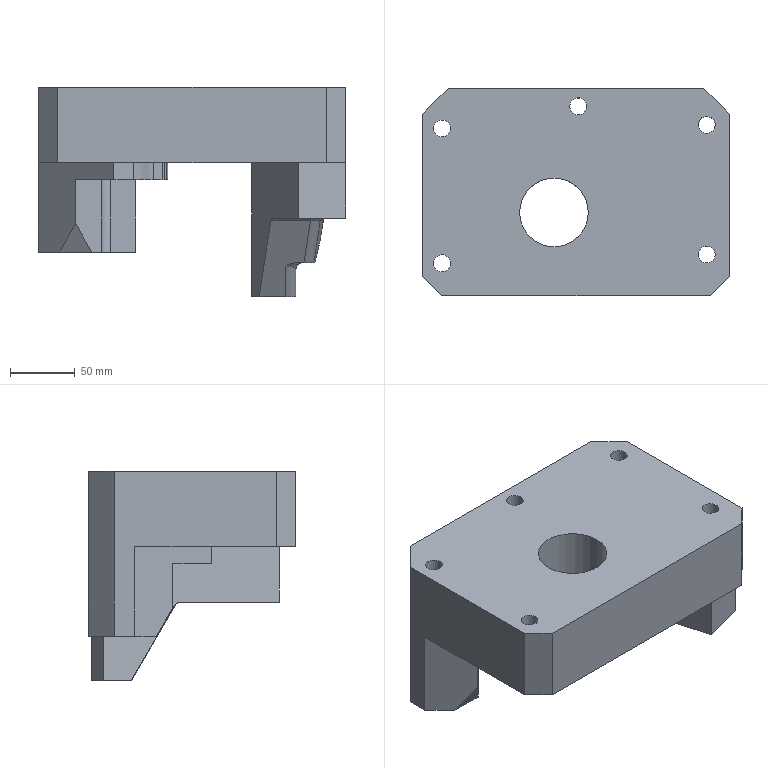Part | NX | features solid 2 | 1 solid | 95 faces | box 237 x 160 x 161.25 mm | volume 2516063 mm3 | plane 47 | cylinder 32 | cone 10 | spline 6 | commonest cylinder face diameters 13 x5 20 x5 8 x4 15 x4 5 x2 8.506 x2